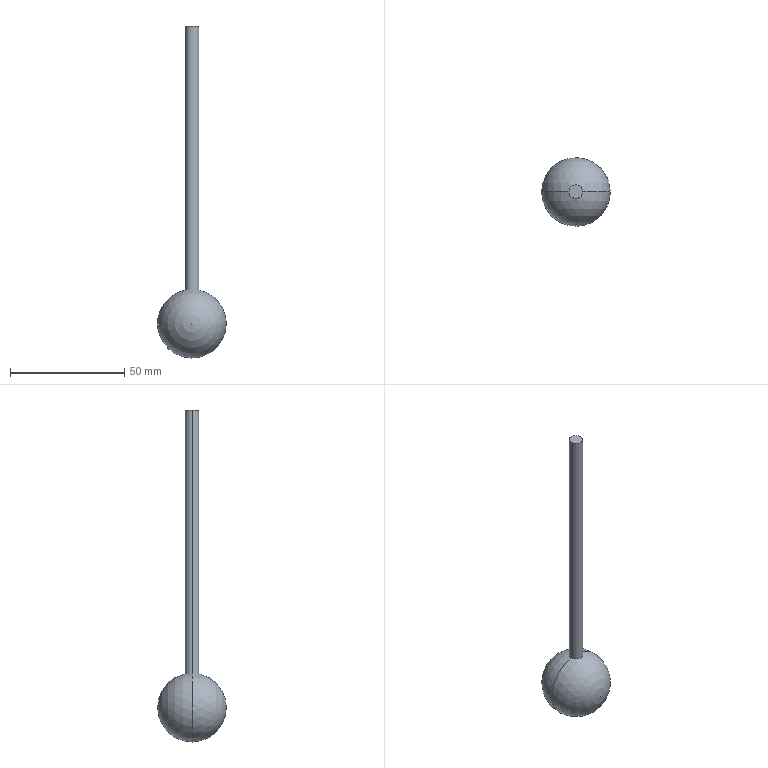Part | SolidWorks | features ICE 1, Revolution 1 | 1 solid | 5 faces | box 30 x 30 x 145 mm | volume 17393 mm3 | cylinder 2 | sphere 2 | plane 1 | commonest cylinder face diameters 6 x2
STEP:
#1=CARTESIAN_POINT('',(3.,0.,130.));
#2=VERTEX_POINT('',#1);
#3=CARTESIAN_POINT('',(-3.,0.,130.));
#4=VERTEX_POINT('',#3);
#5=CARTESIAN_POINT('',(0.,0.,130.));
#6=DIRECTION('',(0.,0.,1.));
#7=DIRECTION('',(1.,0.,0.));
#8=AXIS2_PLACEMENT_3D('',#5,#6,#7);
#9=CIRCLE('',#8,3.);
#10=EDGE_CURVE('',#2,#4,#9,.T.);
#11=ORIENTED_EDGE('',*,*,#10,.F.);
#12=CARTESIAN_POINT('',(3.,0.,14.697));
#13=VERTEX_POINT('',#12);
#14=CARTESIAN_POINT('',(3.,0.,130.));
#15=DIRECTION('',(0.,0.,-1.));
#16=VECTOR('',#15,1000.);
#17=LINE('',#14,#16);
#18=EDGE_CURVE('',#2,#13,#17,.T.);
#19=ORIENTED_EDGE('',*,*,#18,.T.);
#20=CARTESIAN_POINT('',(-3.,0.,14.697));
#21=VERTEX_POINT('',#20);
#22=CARTESIAN_POINT('',(0.,0.,14.697));
#23=DIRECTION('',(0.,0.,1.));
#24=DIRECTION('',(-1.,0.,0.));
#25=AXIS2_PLACEMENT_3D('',#22,#23,#24);
#26=CIRCLE('',#25,3.);
#27=EDGE_CURVE('',#13,#21,#26,.T.);
#28=ORIENTED_EDGE('',*,*,#27,.T.);
#29=CARTESIAN_POINT('',(-3.,0.,130.));
#30=DIRECTION('',(0.,0.,-1.));
#31=VECTOR('',#30,1000.);
#32=LINE('',#29,#31);
#33=EDGE_CURVE('',#4,#21,#32,.T.);
#34=ORIENTED_EDGE('',*,*,#33,.F.);
#35=EDGE_LOOP('',(#11,#19,#28,#34));
#36=FACE_OUTER_BOUND('',#35,.T.);
#37=CARTESIAN_POINT('',(0.,0.,130.));
#38=DIRECTION('',(0.,0.,-1.));
#39=DIRECTION('',(-1.,0.,0.));
#40=AXIS2_PLACEMENT_3D('',#37,#38,#39);
#41=CYLINDRICAL_SURFACE('',#40,3.);
#42=ADVANCED_FACE('',(#36),#41,.T.);
#43=CARTESIAN_POINT('',(0.,0.,-15.));
#44=VERTEX_POINT('',#43);
#45=CARTESIAN_POINT('',(0.,0.,0.));
#46=DIRECTION('',(0.,-1.,0.));
#47=DIRECTION('',(0.,0.,-1.));
#48=AXIS2_PLACEMENT_3D('',#45,#46,#47);
#49=CIRCLE('',#48,15.);
#50=EDGE_CURVE('',#44,#13,#49,.T.);
#51=ORIENTED_EDGE('',*,*,#50,.F.);
#52=CARTESIAN_POINT('',(0.,0.,0.));
#53=DIRECTION('',(0.,1.,0.));
#54=DIRECTION('',(-1.,0.,0.));
#55=AXIS2_PLACEMENT_3D('',#52,#53,#54);
#56=CIRCLE('',#55,15.);
#57=EDGE_CURVE('',#44,#21,#56,.T.);
#58=ORIENTED_EDGE('',*,*,#57,.T.);
#59=ORIENTED_EDGE('',*,*,#27,.F.);
#60=EDGE_LOOP('',(#51,#58,#59));
#61=FACE_OUTER_BOUND('',#60,.T.);
#62=CARTESIAN_POINT('',(0.,0.,0.));
#63=DIRECTION('',(0.,1.,0.));
#64=DIRECTION('',(1.,0.,0.));
#65=AXIS2_PLACEMENT_3D('',#62,#63,#64);
#66=SPHERICAL_SURFACE('',#65,15.);
#67=ADVANCED_FACE('',(#61),#66,.T.);
#68=ORIENTED_EDGE('',*,*,#57,.F.);
#69=ORIENTED_EDGE('',*,*,#50,.T.);
#70=CARTESIAN_POINT('',(0.,0.,14.697));
#71=DIRECTION('',(0.,0.,1.));
#72=DIRECTION('',(-1.,0.,0.));
#73=AXIS2_PLACEMENT_3D('',#70,#71,#72);
#74=CIRCLE('',#73,3.);
#75=EDGE_CURVE('',#21,#13,#74,.T.);
#76=ORIENTED_EDGE('',*,*,#75,.F.);
#77=EDGE_LOOP('',(#68,#69,#76));
#78=FACE_OUTER_BOUND('',#77,.T.);
#79=CARTESIAN_POINT('',(0.,0.,0.));
#80=DIRECTION('',(0.,1.,0.));
#81=DIRECTION('',(1.,0.,0.));
#82=AXIS2_PLACEMENT_3D('',#79,#80,#81);
#83=SPHERICAL_SURFACE('',#82,15.);
#84=ADVANCED_FACE('',(#78),#83,.T.);
#85=ORIENTED_EDGE('',*,*,#18,.F.);
#86=CARTESIAN_POINT('',(0.,0.,130.));
#87=DIRECTION('',(0.,0.,1.));
#88=DIRECTION('',(1.,0.,0.));
#89=AXIS2_PLACEMENT_3D('',#86,#87,#88);
#90=CIRCLE('',#89,3.);
#91=EDGE_CURVE('',#4,#2,#90,.T.);
#92=ORIENTED_EDGE('',*,*,#91,.F.);
#93=ORIENTED_EDGE('',*,*,#33,.T.);
#94=ORIENTED_EDGE('',*,*,#75,.T.);
#95=EDGE_LOOP('',(#85,#92,#93,#94));
#96=FACE_OUTER_BOUND('',#95,.T.);
#97=CARTESIAN_POINT('',(0.,0.,130.));
#98=DIRECTION('',(0.,0.,-1.));
#99=DIRECTION('',(-1.,0.,0.));
#100=AXIS2_PLACEMENT_3D('',#97,#98,#99);
#101=CYLINDRICAL_SURFACE('',#100,3.);
#102=ADVANCED_FACE('',(#96),#101,.T.);
#103=ORIENTED_EDGE('',*,*,#91,.T.);
#104=ORIENTED_EDGE('',*,*,#10,.T.);
#105=EDGE_LOOP('',(#103,#104));
#106=FACE_OUTER_BOUND('',#105,.T.);
#107=CARTESIAN_POINT('',(0.,0.,130.));
#108=DIRECTION('',(0.,0.,1.));
#109=DIRECTION('',(1.,0.,0.));
#110=AXIS2_PLACEMENT_3D('',#107,#108,#109);
#111=PLANE('',#110);
#112=ADVANCED_FACE('',(#106),#111,.T.);
#113=CLOSED_SHELL('',(#42,#67,#84,#102,#112));
#114=MANIFOLD_SOLID_BREP('',#113);
#115=CARTESIAN_POINT('',(0.,0.,0.));
#116=DIRECTION('',(0.,0.,1.));
#117=DIRECTION('',(1.,0.,0.));
#118=AXIS2_PLACEMENT_3D('',#115,#116,#117);
#119=(LENGTH_UNIT()NAMED_UNIT(*)SI_UNIT(.MILLI.,.METRE.));
#120=UNCERTAINTY_MEASURE_WITH_UNIT(LENGTH_MEASURE(0.00001),#119,'','');
#121=(NAMED_UNIT(*)PLANE_ANGLE_UNIT()SI_UNIT($,.RADIAN.));
#122=(NAMED_UNIT(*)SI_UNIT($,.STERADIAN.)SOLID_ANGLE_UNIT());
#123=(GEOMETRIC_REPRESENTATION_CONTEXT(3)GLOBAL_UNCERTAINTY_ASSIGNED_CONTEXT((#120))GLOBAL_UNIT_ASSIGNED_CONTEXT((#119,#121,#122))REPRESENTATION_CONTEXT('',''));
#124=ADVANCED_BREP_SHAPE_REPRESENTATION('',(#114,#118),#123);